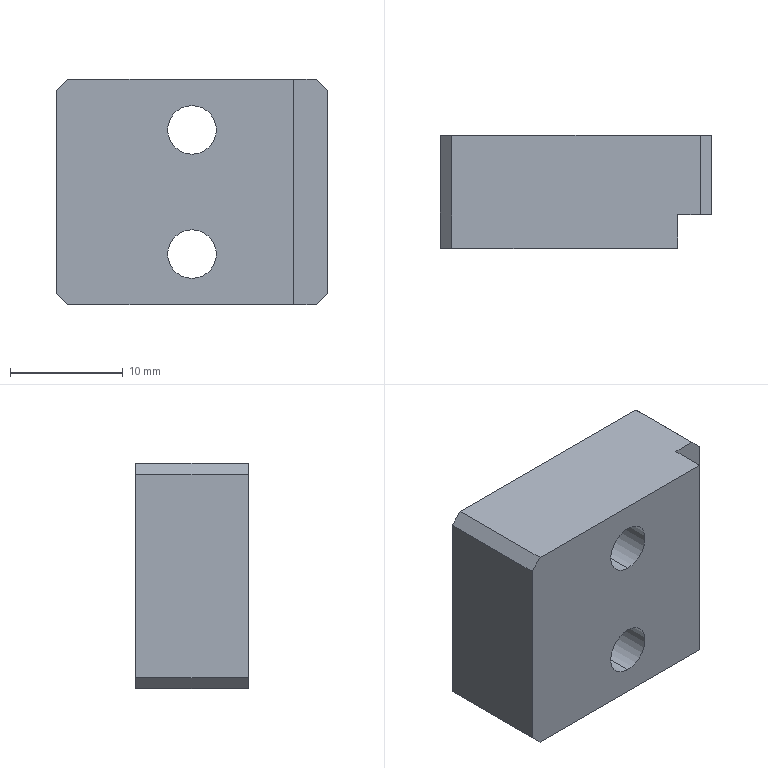Part | STEP file | PN_0059 | 1 solid | 16 faces | box 24 x 10 x 20 mm | volume 4313 mm3 | plane 12 | cylinder 4 | commonest cylinder face diameters 4.3 x4
STEP:
#1=CARTESIAN_POINT('',(0.,0.,0.));
#2=DIRECTION('',(0.,0.,1.));
#3=DIRECTION('',(1.,0.,0.));
#4=AXIS2_PLACEMENT_3D('',#1,#2,#3);
#5=CARTESIAN_POINT('',(0.,0.,7.65));
#6=VERTEX_POINT('',#5);
#7=CARTESIAN_POINT('',(0.,10.,7.65));
#8=VERTEX_POINT('',#7);
#9=CARTESIAN_POINT('',(0.,-43.,7.65));
#10=DIRECTION('',(0.,1.,0.));
#11=VECTOR('',#10,1.);
#12=LINE('',#9,#11);
#13=CARTESIAN_POINT('',(0.,-43.,5.5));
#14=DIRECTION('',(0.,1.,0.));
#15=DIRECTION('',(0.,0.,1.));
#16=AXIS2_PLACEMENT_3D('',#13,#14,#15);
#17=CYLINDRICAL_SURFACE('',#16,2.15);
#18=CARTESIAN_POINT('',(6.283,0.));
#19=DIRECTION('',(0.,1.));
#20=VECTOR('',#19,1.);
#21=LINE('',#18,#20);
#22=(GEOMETRIC_REPRESENTATION_CONTEXT(2)PARAMETRIC_REPRESENTATION_CONTEXT()REPRESENTATION_CONTEXT('',''));
#23=DEFINITIONAL_REPRESENTATION('',(#21),#22);
#24=PCURVE('',#17,#23);
#25=CARTESIAN_POINT('',(0.,-43.,5.5));
#26=DIRECTION('',(0.,1.,0.));
#27=DIRECTION('',(0.,0.,1.));
#28=AXIS2_PLACEMENT_3D('',#25,#26,#27);
#29=CYLINDRICAL_SURFACE('',#28,2.15);
#30=CARTESIAN_POINT('',(0.,0.));
#31=DIRECTION('',(0.,1.));
#32=VECTOR('',#31,1.);
#33=LINE('',#30,#32);
#34=(GEOMETRIC_REPRESENTATION_CONTEXT(2)PARAMETRIC_REPRESENTATION_CONTEXT()REPRESENTATION_CONTEXT('',''));
#35=DEFINITIONAL_REPRESENTATION('',(#33),#34);
#36=PCURVE('',#29,#35);
#37=SURFACE_CURVE('',#12,(#24,#36),.PCURVE_S1.);
#38=EDGE_CURVE('',#6,#8,#37,.T.);
#39=ORIENTED_EDGE('',*,*,#38,.T.);
#40=CARTESIAN_POINT('',(0.,10.,3.35));
#41=VERTEX_POINT('',#40);
#42=CARTESIAN_POINT('',(0.,10.,5.5));
#43=DIRECTION('',(0.,1.,0.));
#44=DIRECTION('',(0.,0.,1.));
#45=AXIS2_PLACEMENT_3D('',#42,#43,#44);
#46=CIRCLE('',#45,2.15);
#47=CARTESIAN_POINT('',(0.,53.));
#48=DIRECTION('',(1.,0.));
#49=VECTOR('',#48,1.);
#50=LINE('',#47,#49);
#51=(GEOMETRIC_REPRESENTATION_CONTEXT(2)PARAMETRIC_REPRESENTATION_CONTEXT()REPRESENTATION_CONTEXT('',''));
#52=DEFINITIONAL_REPRESENTATION('',(#50),#51);
#53=PCURVE('',#17,#52);
#54=CARTESIAN_POINT('',(0.,10.,0.));
#55=DIRECTION('',(0.,1.,0.));
#56=DIRECTION('',(0.,0.,1.));
#57=AXIS2_PLACEMENT_3D('',#54,#55,#56);
#58=PLANE('',#57);
#59=CARTESIAN_POINT('',(5.5,0.));
#60=DIRECTION('',(1.,0.));
#61=AXIS2_PLACEMENT_2D('',#59,#60);
#62=CIRCLE('',#61,2.15);
#63=(GEOMETRIC_REPRESENTATION_CONTEXT(2)PARAMETRIC_REPRESENTATION_CONTEXT()REPRESENTATION_CONTEXT('',''));
#64=DEFINITIONAL_REPRESENTATION('',(#62),#63);
#65=PCURVE('',#58,#64);
#66=SURFACE_CURVE('',#46,(#53,#65),.PCURVE_S1.);
#67=EDGE_CURVE('',#41,#8,#66,.T.);
#68=ORIENTED_EDGE('',*,*,#67,.F.);
#69=CARTESIAN_POINT('',(0.,0.,3.35));
#70=VERTEX_POINT('',#69);
#71=CARTESIAN_POINT('',(0.,-43.,3.35));
#72=DIRECTION('',(0.,1.,0.));
#73=VECTOR('',#72,1.);
#74=LINE('',#71,#73);
#75=CARTESIAN_POINT('',(3.142,0.));
#76=DIRECTION('',(0.,1.));
#77=VECTOR('',#76,1.);
#78=LINE('',#75,#77);
#79=(GEOMETRIC_REPRESENTATION_CONTEXT(2)PARAMETRIC_REPRESENTATION_CONTEXT()REPRESENTATION_CONTEXT('',''));
#80=DEFINITIONAL_REPRESENTATION('',(#78),#79);
#81=PCURVE('',#17,#80);
#82=CARTESIAN_POINT('',(3.142,0.));
#83=DIRECTION('',(0.,1.));
#84=VECTOR('',#83,1.);
#85=LINE('',#82,#84);
#86=(GEOMETRIC_REPRESENTATION_CONTEXT(2)PARAMETRIC_REPRESENTATION_CONTEXT()REPRESENTATION_CONTEXT('',''));
#87=DEFINITIONAL_REPRESENTATION('',(#85),#86);
#88=PCURVE('',#29,#87);
#89=SURFACE_CURVE('',#74,(#81,#88),.PCURVE_S1.);
#90=EDGE_CURVE('',#70,#41,#89,.T.);
#91=ORIENTED_EDGE('',*,*,#90,.F.);
#92=CARTESIAN_POINT('',(0.,0.,5.5));
#93=DIRECTION('',(0.,1.,0.));
#94=DIRECTION('',(0.,0.,1.));
#95=AXIS2_PLACEMENT_3D('',#92,#93,#94);
#96=CIRCLE('',#95,2.15);
#97=CARTESIAN_POINT('',(0.,43.));
#98=DIRECTION('',(1.,0.));
#99=VECTOR('',#98,1.);
#100=LINE('',#97,#99);
#101=(GEOMETRIC_REPRESENTATION_CONTEXT(2)PARAMETRIC_REPRESENTATION_CONTEXT()REPRESENTATION_CONTEXT('',''));
#102=DEFINITIONAL_REPRESENTATION('',(#100),#101);
#103=PCURVE('',#17,#102);
#104=CARTESIAN_POINT('',(0.,0.,0.));
#105=DIRECTION('',(0.,1.,0.));
#106=DIRECTION('',(0.,0.,1.));
#107=AXIS2_PLACEMENT_3D('',#104,#105,#106);
#108=PLANE('',#107);
#109=CARTESIAN_POINT('',(5.5,0.));
#110=DIRECTION('',(1.,0.));
#111=AXIS2_PLACEMENT_2D('',#109,#110);
#112=CIRCLE('',#111,2.15);
#113=(GEOMETRIC_REPRESENTATION_CONTEXT(2)PARAMETRIC_REPRESENTATION_CONTEXT()REPRESENTATION_CONTEXT('',''));
#114=DEFINITIONAL_REPRESENTATION('',(#112),#113);
#115=PCURVE('',#108,#114);
#116=SURFACE_CURVE('',#96,(#103,#115),.PCURVE_S1.);
#117=EDGE_CURVE('',#70,#6,#116,.T.);
#118=ORIENTED_EDGE('',*,*,#117,.T.);
#119=EDGE_LOOP('',(#39,#68,#91,#118));
#120=FACE_BOUND('',#119,.F.);
#121=ADVANCED_FACE('',(#120),#17,.F.);
#122=CARTESIAN_POINT('',(0.,0.,-3.35));
#123=VERTEX_POINT('',#122);
#124=CARTESIAN_POINT('',(0.,10.,-3.35));
#125=VERTEX_POINT('',#124);
#126=CARTESIAN_POINT('',(0.,-43.,-3.35));
#127=DIRECTION('',(0.,1.,0.));
#128=VECTOR('',#127,1.);
#129=LINE('',#126,#128);
#130=CARTESIAN_POINT('',(0.,-43.,-5.5));
#131=DIRECTION('',(0.,1.,0.));
#132=DIRECTION('',(0.,0.,1.));
#133=AXIS2_PLACEMENT_3D('',#130,#131,#132);
#134=CYLINDRICAL_SURFACE('',#133,2.15);
#135=CARTESIAN_POINT('',(6.283,0.));
#136=DIRECTION('',(0.,1.));
#137=VECTOR('',#136,1.);
#138=LINE('',#135,#137);
#139=(GEOMETRIC_REPRESENTATION_CONTEXT(2)PARAMETRIC_REPRESENTATION_CONTEXT()REPRESENTATION_CONTEXT('',''));
#140=DEFINITIONAL_REPRESENTATION('',(#138),#139);
#141=PCURVE('',#134,#140);
#142=CARTESIAN_POINT('',(0.,-43.,-5.5));
#143=DIRECTION('',(0.,1.,0.));
#144=DIRECTION('',(0.,0.,1.));
#145=AXIS2_PLACEMENT_3D('',#142,#143,#144);
#146=CYLINDRICAL_SURFACE('',#145,2.15);
#147=CARTESIAN_POINT('',(0.,0.));
#148=DIRECTION('',(0.,1.));
#149=VECTOR('',#148,1.);
#150=LINE('',#147,#149);
#151=(GEOMETRIC_REPRESENTATION_CONTEXT(2)PARAMETRIC_REPRESENTATION_CONTEXT()REPRESENTATION_CONTEXT('',''));
#152=DEFINITIONAL_REPRESENTATION('',(#150),#151);
#153=PCURVE('',#146,#152);
#154=SURFACE_CURVE('',#129,(#141,#153),.PCURVE_S1.);
#155=EDGE_CURVE('',#123,#125,#154,.T.);
#156=ORIENTED_EDGE('',*,*,#155,.T.);
#157=CARTESIAN_POINT('',(0.,10.,-7.65));
#158=VERTEX_POINT('',#157);
#159=CARTESIAN_POINT('',(0.,10.,-5.5));
#160=DIRECTION('',(0.,1.,0.));
#161=DIRECTION('',(0.,0.,1.));
#162=AXIS2_PLACEMENT_3D('',#159,#160,#161);
#163=CIRCLE('',#162,2.15);
#164=CARTESIAN_POINT('',(0.,53.));
#165=DIRECTION('',(1.,0.));
#166=VECTOR('',#165,1.);
#167=LINE('',#164,#166);
#168=(GEOMETRIC_REPRESENTATION_CONTEXT(2)PARAMETRIC_REPRESENTATION_CONTEXT()REPRESENTATION_CONTEXT('',''));
#169=DEFINITIONAL_REPRESENTATION('',(#167),#168);
#170=PCURVE('',#134,#169);
#171=CARTESIAN_POINT('',(-5.5,0.));
#172=DIRECTION('',(1.,0.));
#173=AXIS2_PLACEMENT_2D('',#171,#172);
#174=CIRCLE('',#173,2.15);
#175=(GEOMETRIC_REPRESENTATION_CONTEXT(2)PARAMETRIC_REPRESENTATION_CONTEXT()REPRESENTATION_CONTEXT('',''));
#176=DEFINITIONAL_REPRESENTATION('',(#174),#175);
#177=PCURVE('',#58,#176);
#178=SURFACE_CURVE('',#163,(#170,#177),.PCURVE_S1.);
#179=EDGE_CURVE('',#158,#125,#178,.T.);
#180=ORIENTED_EDGE('',*,*,#179,.F.);
#181=CARTESIAN_POINT('',(0.,0.,-7.65));
#182=VERTEX_POINT('',#181);
#183=CARTESIAN_POINT('',(0.,-43.,-7.65));
#184=DIRECTION('',(0.,1.,0.));
#185=VECTOR('',#184,1.);
#186=LINE('',#183,#185);
#187=CARTESIAN_POINT('',(3.142,0.));
#188=DIRECTION('',(0.,1.));
#189=VECTOR('',#188,1.);
#190=LINE('',#187,#189);
#191=(GEOMETRIC_REPRESENTATION_CONTEXT(2)PARAMETRIC_REPRESENTATION_CONTEXT()REPRESENTATION_CONTEXT('',''));
#192=DEFINITIONAL_REPRESENTATION('',(#190),#191);
#193=PCURVE('',#134,#192);
#194=CARTESIAN_POINT('',(3.142,0.));
#195=DIRECTION('',(0.,1.));
#196=VECTOR('',#195,1.);
#197=LINE('',#194,#196);
#198=(GEOMETRIC_REPRESENTATION_CONTEXT(2)PARAMETRIC_REPRESENTATION_CONTEXT()REPRESENTATION_CONTEXT('',''));
#199=DEFINITIONAL_REPRESENTATION('',(#197),#198);
#200=PCURVE('',#146,#199);
#201=SURFACE_CURVE('',#186,(#193,#200),.PCURVE_S1.);
#202=EDGE_CURVE('',#182,#158,#201,.T.);
#203=ORIENTED_EDGE('',*,*,#202,.F.);
#204=CARTESIAN_POINT('',(0.,0.,-5.5));
#205=DIRECTION('',(0.,1.,0.));
#206=DIRECTION('',(0.,0.,1.));
#207=AXIS2_PLACEMENT_3D('',#204,#205,#206);
#208=CIRCLE('',#207,2.15);
#209=CARTESIAN_POINT('',(0.,43.));
#210=DIRECTION('',(1.,0.));
#211=VECTOR('',#210,1.);
#212=LINE('',#209,#211);
#213=(GEOMETRIC_REPRESENTATION_CONTEXT(2)PARAMETRIC_REPRESENTATION_CONTEXT()REPRESENTATION_CONTEXT('',''));
#214=DEFINITIONAL_REPRESENTATION('',(#212),#213);
#215=PCURVE('',#134,#214);
#216=CARTESIAN_POINT('',(-5.5,0.));
#217=DIRECTION('',(1.,0.));
#218=AXIS2_PLACEMENT_2D('',#216,#217);
#219=CIRCLE('',#218,2.15);
#220=(GEOMETRIC_REPRESENTATION_CONTEXT(2)PARAMETRIC_REPRESENTATION_CONTEXT()REPRESENTATION_CONTEXT('',''));
#221=DEFINITIONAL_REPRESENTATION('',(#219),#220);
#222=PCURVE('',#108,#221);
#223=SURFACE_CURVE('',#208,(#215,#222),.PCURVE_S1.);
#224=EDGE_CURVE('',#182,#123,#223,.T.);
#225=ORIENTED_EDGE('',*,*,#224,.T.);
#226=EDGE_LOOP('',(#156,#180,#203,#225));
#227=FACE_BOUND('',#226,.F.);
#228=ADVANCED_FACE('',(#227),#134,.F.);
#229=CARTESIAN_POINT('',(12.,3.,-9.));
#230=VERTEX_POINT('',#229);
#231=CARTESIAN_POINT('',(12.,3.,9.));
#232=VERTEX_POINT('',#231);
#233=CARTESIAN_POINT('',(12.,3.,-29.));
#234=DIRECTION('',(0.,0.,1.));
#235=VECTOR('',#234,1.);
#236=LINE('',#233,#235);
#237=CARTESIAN_POINT('',(12.,10.,-10.));
#238=DIRECTION('',(-1.,0.,0.));
#239=DIRECTION('',(0.,0.,1.));
#240=AXIS2_PLACEMENT_3D('',#237,#238,#239);
#241=PLANE('',#240);
#242=CARTESIAN_POINT('',(-19.,-7.));
#243=DIRECTION('',(1.,0.));
#244=VECTOR('',#243,1.);
#245=LINE('',#242,#244);
#246=(GEOMETRIC_REPRESENTATION_CONTEXT(2)PARAMETRIC_REPRESENTATION_CONTEXT()REPRESENTATION_CONTEXT('',''));
#247=DEFINITIONAL_REPRESENTATION('',(#245),#246);
#248=PCURVE('',#241,#247);
#249=CARTESIAN_POINT('',(12.,3.,-29.));
#250=DIRECTION('',(0.,1.,0.));
#251=DIRECTION('',(-1.,0.,0.));
#252=AXIS2_PLACEMENT_3D('',#249,#250,#251);
#253=PLANE('',#252);
#254=CARTESIAN_POINT('',(0.,0.));
#255=DIRECTION('',(0.,1.));
#256=VECTOR('',#255,1.);
#257=LINE('',#254,#256);
#258=(GEOMETRIC_REPRESENTATION_CONTEXT(2)PARAMETRIC_REPRESENTATION_CONTEXT()REPRESENTATION_CONTEXT('',''));
#259=DEFINITIONAL_REPRESENTATION('',(#257),#258);
#260=PCURVE('',#253,#259);
#261=SURFACE_CURVE('',#236,(#248,#260),.PCURVE_S1.);
#262=EDGE_CURVE('',#230,#232,#261,.T.);
#263=ORIENTED_EDGE('',*,*,#262,.F.);
#264=CARTESIAN_POINT('',(12.,10.,-9.));
#265=VERTEX_POINT('',#264);
#266=CARTESIAN_POINT('',(12.,10.,-9.));
#267=DIRECTION('',(0.,1.,0.));
#268=VECTOR('',#267,1.);
#269=LINE('',#266,#268);
#270=CARTESIAN_POINT('',(1.,0.));
#271=DIRECTION('',(0.,1.));
#272=VECTOR('',#271,1.);
#273=LINE('',#270,#272);
#274=(GEOMETRIC_REPRESENTATION_CONTEXT(2)PARAMETRIC_REPRESENTATION_CONTEXT()REPRESENTATION_CONTEXT('',''));
#275=DEFINITIONAL_REPRESENTATION('',(#273),#274);
#276=PCURVE('',#241,#275);
#277=CARTESIAN_POINT('',(11.,10.,-10.));
#278=DIRECTION('',(-0.7071,0.,0.7071));
#279=DIRECTION('',(0.,-1.,0.));
#280=AXIS2_PLACEMENT_3D('',#277,#278,#279);
#281=PLANE('',#280);
#282=CARTESIAN_POINT('',(0.,1.414));
#283=DIRECTION('',(-1.,0.));
#284=VECTOR('',#283,1.);
#285=LINE('',#282,#284);
#286=(GEOMETRIC_REPRESENTATION_CONTEXT(2)PARAMETRIC_REPRESENTATION_CONTEXT()REPRESENTATION_CONTEXT('',''));
#287=DEFINITIONAL_REPRESENTATION('',(#285),#286);
#288=PCURVE('',#281,#287);
#289=SURFACE_CURVE('',#269,(#276,#288),.PCURVE_S1.);
#290=EDGE_CURVE('',#230,#265,#289,.T.);
#291=ORIENTED_EDGE('',*,*,#290,.T.);
#292=CARTESIAN_POINT('',(12.,10.,9.));
#293=VERTEX_POINT('',#292);
#294=CARTESIAN_POINT('',(12.,10.,-10.));
#295=DIRECTION('',(0.,0.,-1.));
#296=VECTOR('',#295,1.);
#297=LINE('',#294,#296);
#298=CARTESIAN_POINT('',(0.,0.));
#299=DIRECTION('',(-1.,0.));
#300=VECTOR('',#299,1.);
#301=LINE('',#298,#300);
#302=(GEOMETRIC_REPRESENTATION_CONTEXT(2)PARAMETRIC_REPRESENTATION_CONTEXT()REPRESENTATION_CONTEXT('',''));
#303=DEFINITIONAL_REPRESENTATION('',(#301),#302);
#304=PCURVE('',#241,#303);
#305=CARTESIAN_POINT('',(-10.,12.));
#306=DIRECTION('',(-1.,0.));
#307=VECTOR('',#306,1.);
#308=LINE('',#305,#307);
#309=(GEOMETRIC_REPRESENTATION_CONTEXT(2)PARAMETRIC_REPRESENTATION_CONTEXT()REPRESENTATION_CONTEXT('',''));
#310=DEFINITIONAL_REPRESENTATION('',(#308),#309);
#311=PCURVE('',#58,#310);
#312=SURFACE_CURVE('',#297,(#304,#311),.PCURVE_S1.);
#313=EDGE_CURVE('',#293,#265,#312,.T.);
#314=ORIENTED_EDGE('',*,*,#313,.F.);
#315=CARTESIAN_POINT('',(12.,10.,9.));
#316=DIRECTION('',(0.,-1.,0.));
#317=VECTOR('',#316,1.);
#318=LINE('',#315,#317);
#319=CARTESIAN_POINT('',(19.,0.));
#320=DIRECTION('',(0.,-1.));
#321=VECTOR('',#320,1.);
#322=LINE('',#319,#321);
#323=(GEOMETRIC_REPRESENTATION_CONTEXT(2)PARAMETRIC_REPRESENTATION_CONTEXT()REPRESENTATION_CONTEXT('',''));
#324=DEFINITIONAL_REPRESENTATION('',(#322),#323);
#325=PCURVE('',#241,#324);
#326=CARTESIAN_POINT('',(12.,10.,9.));
#327=DIRECTION('',(-0.7071,0.,-0.7071));
#328=DIRECTION('',(0.,-1.,0.));
#329=AXIS2_PLACEMENT_3D('',#326,#327,#328);
#330=PLANE('',#329);
#331=CARTESIAN_POINT('',(0.,0.));
#332=DIRECTION('',(1.,0.));
#333=VECTOR('',#332,1.);
#334=LINE('',#331,#333);
#335=(GEOMETRIC_REPRESENTATION_CONTEXT(2)PARAMETRIC_REPRESENTATION_CONTEXT()REPRESENTATION_CONTEXT('',''));
#336=DEFINITIONAL_REPRESENTATION('',(#334),#335);
#337=PCURVE('',#330,#336);
#338=SURFACE_CURVE('',#318,(#325,#337),.PCURVE_S1.);
#339=EDGE_CURVE('',#293,#232,#338,.T.);
#340=ORIENTED_EDGE('',*,*,#339,.T.);
#341=EDGE_LOOP('',(#263,#291,#314,#340));
#342=FACE_BOUND('',#341,.T.);
#343=ADVANCED_FACE('',(#342),#241,.F.);
#344=CARTESIAN_POINT('',(9.,0.,-10.));
#345=VERTEX_POINT('',#344);
#346=CARTESIAN_POINT('',(-11.,0.,-10.));
#347=VERTEX_POINT('',#346);
#348=CARTESIAN_POINT('',(-12.,0.,-10.));
#349=DIRECTION('',(-1.,0.,0.));
#350=VECTOR('',#349,1.);
#351=LINE('',#348,#350);
#352=CARTESIAN_POINT('',(-12.,10.,-10.));
#353=DIRECTION('',(0.,0.,1.));
#354=DIRECTION('',(1.,0.,0.));
#355=AXIS2_PLACEMENT_3D('',#352,#353,#354);
#356=PLANE('',#355);
#357=CARTESIAN_POINT('',(0.,-10.));
#358=DIRECTION('',(-1.,0.));
#359=VECTOR('',#358,1.);
#360=LINE('',#357,#359);
#361=(GEOMETRIC_REPRESENTATION_CONTEXT(2)PARAMETRIC_REPRESENTATION_CONTEXT()REPRESENTATION_CONTEXT('',''));
#362=DEFINITIONAL_REPRESENTATION('',(#360),#361);
#363=PCURVE('',#356,#362);
#364=CARTESIAN_POINT('',(-10.,-12.));
#365=DIRECTION('',(0.,-1.));
#366=VECTOR('',#365,1.);
#367=LINE('',#364,#366);
#368=(GEOMETRIC_REPRESENTATION_CONTEXT(2)PARAMETRIC_REPRESENTATION_CONTEXT()REPRESENTATION_CONTEXT('',''));
#369=DEFINITIONAL_REPRESENTATION('',(#367),#368);
#370=PCURVE('',#108,#369);
#371=SURFACE_CURVE('',#351,(#363,#370),.PCURVE_S1.);
#372=EDGE_CURVE('',#345,#347,#371,.T.);
#373=ORIENTED_EDGE('',*,*,#372,.T.);
#374=CARTESIAN_POINT('',(-11.,10.,-10.));
#375=VERTEX_POINT('',#374);
#376=CARTESIAN_POINT('',(-11.,10.,-10.));
#377=DIRECTION('',(0.,1.,0.));
#378=VECTOR('',#377,1.);
#379=LINE('',#376,#378);
#380=CARTESIAN_POINT('',(1.,0.));
#381=DIRECTION('',(0.,1.));
#382=VECTOR('',#381,1.);
#383=LINE('',#380,#382);
#384=(GEOMETRIC_REPRESENTATION_CONTEXT(2)PARAMETRIC_REPRESENTATION_CONTEXT()REPRESENTATION_CONTEXT('',''));
#385=DEFINITIONAL_REPRESENTATION('',(#383),#384);
#386=PCURVE('',#356,#385);
#387=CARTESIAN_POINT('',(-12.,10.,-9.));
#388=DIRECTION('',(0.7071,0.,0.7071));
#389=DIRECTION('',(0.,-1.,0.));
#390=AXIS2_PLACEMENT_3D('',#387,#388,#389);
#391=PLANE('',#390);
#392=CARTESIAN_POINT('',(0.,1.414));
#393=DIRECTION('',(-1.,0.));
#394=VECTOR('',#393,1.);
#395=LINE('',#392,#394);
#396=(GEOMETRIC_REPRESENTATION_CONTEXT(2)PARAMETRIC_REPRESENTATION_CONTEXT()REPRESENTATION_CONTEXT('',''));
#397=DEFINITIONAL_REPRESENTATION('',(#395),#396);
#398=PCURVE('',#391,#397);
#399=SURFACE_CURVE('',#379,(#386,#398),.PCURVE_S1.);
#400=EDGE_CURVE('',#347,#375,#399,.T.);
#401=ORIENTED_EDGE('',*,*,#400,.T.);
#402=CARTESIAN_POINT('',(11.,10.,-10.));
#403=VERTEX_POINT('',#402);
#404=CARTESIAN_POINT('',(-12.,10.,-10.));
#405=DIRECTION('',(-1.,0.,0.));
#406=VECTOR('',#405,1.);
#407=LINE('',#404,#406);
#408=CARTESIAN_POINT('',(0.,0.));
#409=DIRECTION('',(-1.,0.));
#410=VECTOR('',#409,1.);
#411=LINE('',#408,#410);
#412=(GEOMETRIC_REPRESENTATION_CONTEXT(2)PARAMETRIC_REPRESENTATION_CONTEXT()REPRESENTATION_CONTEXT('',''));
#413=DEFINITIONAL_REPRESENTATION('',(#411),#412);
#414=PCURVE('',#356,#413);
#415=CARTESIAN_POINT('',(-10.,-12.));
#416=DIRECTION('',(0.,-1.));
#417=VECTOR('',#416,1.);
#418=LINE('',#415,#417);
#419=(GEOMETRIC_REPRESENTATION_CONTEXT(2)PARAMETRIC_REPRESENTATION_CONTEXT()REPRESENTATION_CONTEXT('',''));
#420=DEFINITIONAL_REPRESENTATION('',(#418),#419);
#421=PCURVE('',#58,#420);
#422=SURFACE_CURVE('',#407,(#414,#421),.PCURVE_S1.);
#423=EDGE_CURVE('',#403,#375,#422,.T.);
#424=ORIENTED_EDGE('',*,*,#423,.F.);
#425=CARTESIAN_POINT('',(11.,3.,-10.));
#426=VERTEX_POINT('',#425);
#427=CARTESIAN_POINT('',(11.,10.,-10.));
#428=DIRECTION('',(0.,-1.,0.));
#429=VECTOR('',#428,1.);
#430=LINE('',#427,#429);
#431=CARTESIAN_POINT('',(23.,0.));
#432=DIRECTION('',(0.,-1.));
#433=VECTOR('',#432,1.);
#434=LINE('',#431,#433);
#435=(GEOMETRIC_REPRESENTATION_CONTEXT(2)PARAMETRIC_REPRESENTATION_CONTEXT()REPRESENTATION_CONTEXT('',''));
#436=DEFINITIONAL_REPRESENTATION('',(#434),#435);
#437=PCURVE('',#356,#436);
#438=CARTESIAN_POINT('',(0.,0.));
#439=DIRECTION('',(1.,0.));
#440=VECTOR('',#439,1.);
#441=LINE('',#438,#440);
#442=(GEOMETRIC_REPRESENTATION_CONTEXT(2)PARAMETRIC_REPRESENTATION_CONTEXT()REPRESENTATION_CONTEXT('',''));
#443=DEFINITIONAL_REPRESENTATION('',(#441),#442);
#444=PCURVE('',#281,#443);
#445=SURFACE_CURVE('',#430,(#437,#444),.PCURVE_S1.);
#446=EDGE_CURVE('',#403,#426,#445,.T.);
#447=ORIENTED_EDGE('',*,*,#446,.T.);
#448=CARTESIAN_POINT('',(9.,3.,-10.));
#449=VERTEX_POINT('',#448);
#450=CARTESIAN_POINT('',(-12.,3.,-10.));
#451=DIRECTION('',(-1.,0.,0.));
#452=VECTOR('',#451,1.);
#453=LINE('',#450,#452);
#454=CARTESIAN_POINT('',(0.,-7.));
#455=DIRECTION('',(-1.,0.));
#456=VECTOR('',#455,1.);
#457=LINE('',#454,#456);
#458=(GEOMETRIC_REPRESENTATION_CONTEXT(2)PARAMETRIC_REPRESENTATION_CONTEXT()REPRESENTATION_CONTEXT('',''));
#459=DEFINITIONAL_REPRESENTATION('',(#457),#458);
#460=PCURVE('',#356,#459);
#461=CARTESIAN_POINT('',(24.,19.));
#462=DIRECTION('',(1.,0.));
#463=VECTOR('',#462,1.);
#464=LINE('',#461,#463);
#465=(GEOMETRIC_REPRESENTATION_CONTEXT(2)PARAMETRIC_REPRESENTATION_CONTEXT()REPRESENTATION_CONTEXT('',''));
#466=DEFINITIONAL_REPRESENTATION('',(#464),#465);
#467=PCURVE('',#253,#466);
#468=SURFACE_CURVE('',#453,(#460,#467),.PCURVE_S1.);
#469=EDGE_CURVE('',#426,#449,#468,.T.);
#470=ORIENTED_EDGE('',*,*,#469,.T.);
#471=CARTESIAN_POINT('',(9.,10.,-10.));
#472=DIRECTION('',(0.,-1.,0.));
#473=VECTOR('',#472,1.);
#474=LINE('',#471,#473);
#475=CARTESIAN_POINT('',(21.,0.));
#476=DIRECTION('',(0.,-1.));
#477=VECTOR('',#476,1.);
#478=LINE('',#475,#477);
#479=(GEOMETRIC_REPRESENTATION_CONTEXT(2)PARAMETRIC_REPRESENTATION_CONTEXT()REPRESENTATION_CONTEXT('',''));
#480=DEFINITIONAL_REPRESENTATION('',(#478),#479);
#481=PCURVE('',#356,#480);
#482=CARTESIAN_POINT('',(9.,0.,-29.));
#483=DIRECTION('',(-1.,0.,0.));
#484=DIRECTION('',(0.,0.,1.));
#485=AXIS2_PLACEMENT_3D('',#482,#483,#484);
#486=PLANE('',#485);
#487=CARTESIAN_POINT('',(19.,10.));
#488=DIRECTION('',(0.,-1.));
#489=VECTOR('',#488,1.);
#490=LINE('',#487,#489);
#491=(GEOMETRIC_REPRESENTATION_CONTEXT(2)PARAMETRIC_REPRESENTATION_CONTEXT()REPRESENTATION_CONTEXT('',''));
#492=DEFINITIONAL_REPRESENTATION('',(#490),#491);
#493=PCURVE('',#486,#492);
#494=SURFACE_CURVE('',#474,(#481,#493),.PCURVE_S1.);
#495=EDGE_CURVE('',#449,#345,#494,.T.);
#496=ORIENTED_EDGE('',*,*,#495,.T.);
#497=EDGE_LOOP('',(#373,#401,#424,#447,#470,#496));
#498=FACE_BOUND('',#497,.T.);
#499=ADVANCED_FACE('',(#498),#356,.F.);
#500=CARTESIAN_POINT('',(-12.,10.,-9.));
#501=VERTEX_POINT('',#500);
#502=CARTESIAN_POINT('',(-12.,10.,9.));
#503=VERTEX_POINT('',#502);
#504=CARTESIAN_POINT('',(-12.,10.,-10.));
#505=DIRECTION('',(0.,0.,1.));
#506=VECTOR('',#505,1.);
#507=LINE('',#504,#506);
#508=CARTESIAN_POINT('',(-12.,10.,-10.));
#509=DIRECTION('',(1.,0.,0.));
#510=DIRECTION('',(0.,0.,-1.));
#511=AXIS2_PLACEMENT_3D('',#508,#509,#510);
#512=PLANE('',#511);
#513=CARTESIAN_POINT('',(0.,0.));
#514=DIRECTION('',(-1.,0.));
#515=VECTOR('',#514,1.);
#516=LINE('',#513,#515);
#517=(GEOMETRIC_REPRESENTATION_CONTEXT(2)PARAMETRIC_REPRESENTATION_CONTEXT()REPRESENTATION_CONTEXT('',''));
#518=DEFINITIONAL_REPRESENTATION('',(#516),#517);
#519=PCURVE('',#512,#518);
#520=CARTESIAN_POINT('',(-10.,-12.));
#521=DIRECTION('',(1.,0.));
#522=VECTOR('',#521,1.);
#523=LINE('',#520,#522);
#524=(GEOMETRIC_REPRESENTATION_CONTEXT(2)PARAMETRIC_REPRESENTATION_CONTEXT()REPRESENTATION_CONTEXT('',''));
#525=DEFINITIONAL_REPRESENTATION('',(#523),#524);
#526=PCURVE('',#58,#525);
#527=SURFACE_CURVE('',#507,(#519,#526),.PCURVE_S1.);
#528=EDGE_CURVE('',#501,#503,#527,.T.);
#529=ORIENTED_EDGE('',*,*,#528,.F.);
#530=CARTESIAN_POINT('',(-12.,0.,-9.));
#531=VERTEX_POINT('',#530);
#532=CARTESIAN_POINT('',(-12.,10.,-9.));
#533=DIRECTION('',(0.,-1.,0.));
#534=VECTOR('',#533,1.);
#535=LINE('',#532,#534);
#536=CARTESIAN_POINT('',(-1.,0.));
#537=DIRECTION('',(0.,-1.));
#538=VECTOR('',#537,1.);
#539=LINE('',#536,#538);
#540=(GEOMETRIC_REPRESENTATION_CONTEXT(2)PARAMETRIC_REPRESENTATION_CONTEXT()REPRESENTATION_CONTEXT('',''));
#541=DEFINITIONAL_REPRESENTATION('',(#539),#540);
#542=PCURVE('',#512,#541);
#543=CARTESIAN_POINT('',(0.,0.));
#544=DIRECTION('',(1.,0.));
#545=VECTOR('',#544,1.);
#546=LINE('',#543,#545);
#547=(GEOMETRIC_REPRESENTATION_CONTEXT(2)PARAMETRIC_REPRESENTATION_CONTEXT()REPRESENTATION_CONTEXT('',''));
#548=DEFINITIONAL_REPRESENTATION('',(#546),#547);
#549=PCURVE('',#391,#548);
#550=SURFACE_CURVE('',#535,(#542,#549),.PCURVE_S1.);
#551=EDGE_CURVE('',#501,#531,#550,.T.);
#552=ORIENTED_EDGE('',*,*,#551,.T.);
#553=CARTESIAN_POINT('',(-12.,0.,9.));
#554=VERTEX_POINT('',#553);
#555=CARTESIAN_POINT('',(-12.,0.,-10.));
#556=DIRECTION('',(0.,0.,1.));
#557=VECTOR('',#556,1.);
#558=LINE('',#555,#557);
#559=CARTESIAN_POINT('',(0.,-10.));
#560=DIRECTION('',(-1.,0.));
#561=VECTOR('',#560,1.);
#562=LINE('',#559,#561);
#563=(GEOMETRIC_REPRESENTATION_CONTEXT(2)PARAMETRIC_REPRESENTATION_CONTEXT()REPRESENTATION_CONTEXT('',''));
#564=DEFINITIONAL_REPRESENTATION('',(#562),#563);
#565=PCURVE('',#512,#564);
#566=CARTESIAN_POINT('',(-10.,-12.));
#567=DIRECTION('',(1.,0.));
#568=VECTOR('',#567,1.);
#569=LINE('',#566,#568);
#570=(GEOMETRIC_REPRESENTATION_CONTEXT(2)PARAMETRIC_REPRESENTATION_CONTEXT()REPRESENTATION_CONTEXT('',''));
#571=DEFINITIONAL_REPRESENTATION('',(#569),#570);
#572=PCURVE('',#108,#571);
#573=SURFACE_CURVE('',#558,(#565,#572),.PCURVE_S1.);
#574=EDGE_CURVE('',#531,#554,#573,.T.);
#575=ORIENTED_EDGE('',*,*,#574,.T.);
#576=CARTESIAN_POINT('',(-12.,10.,9.));
#577=DIRECTION('',(0.,1.,0.));
#578=VECTOR('',#577,1.);
#579=LINE('',#576,#578);
#580=CARTESIAN_POINT('',(-19.,0.));
#581=DIRECTION('',(0.,1.));
#582=VECTOR('',#581,1.);
#583=LINE('',#580,#582);
#584=(GEOMETRIC_REPRESENTATION_CONTEXT(2)PARAMETRIC_REPRESENTATION_CONTEXT()REPRESENTATION_CONTEXT('',''));
#585=DEFINITIONAL_REPRESENTATION('',(#583),#584);
#586=PCURVE('',#512,#585);
#587=CARTESIAN_POINT('',(-11.,10.,10.));
#588=DIRECTION('',(0.7071,0.,-0.7071));
#589=DIRECTION('',(0.,-1.,0.));
#590=AXIS2_PLACEMENT_3D('',#587,#588,#589);
#591=PLANE('',#590);
#592=CARTESIAN_POINT('',(0.,1.414));
#593=DIRECTION('',(-1.,0.));
#594=VECTOR('',#593,1.);
#595=LINE('',#592,#594);
#596=(GEOMETRIC_REPRESENTATION_CONTEXT(2)PARAMETRIC_REPRESENTATION_CONTEXT()REPRESENTATION_CONTEXT('',''));
#597=DEFINITIONAL_REPRESENTATION('',(#595),#596);
#598=PCURVE('',#591,#597);
#599=SURFACE_CURVE('',#579,(#586,#598),.PCURVE_S1.);
#600=EDGE_CURVE('',#554,#503,#599,.T.);
#601=ORIENTED_EDGE('',*,*,#600,.T.);
#602=EDGE_LOOP('',(#529,#552,#575,#601));
#603=FACE_BOUND('',#602,.T.);
#604=ADVANCED_FACE('',(#603),#512,.F.);
#605=CARTESIAN_POINT('',(11.,3.,10.));
#606=VERTEX_POINT('',#605);
#607=CARTESIAN_POINT('',(9.,3.,10.));
#608=VERTEX_POINT('',#607);
#609=CARTESIAN_POINT('',(12.,3.,10.));
#610=DIRECTION('',(-1.,0.,0.));
#611=VECTOR('',#610,1.);
#612=LINE('',#609,#611);
#613=CARTESIAN_POINT('',(-12.,10.,10.));
#614=DIRECTION('',(0.,0.,-1.));
#615=DIRECTION('',(-1.,0.,0.));
#616=AXIS2_PLACEMENT_3D('',#613,#614,#615);
#617=PLANE('',#616);
#618=CARTESIAN_POINT('',(-24.,-7.));
#619=DIRECTION('',(1.,0.));
#620=VECTOR('',#619,1.);
#621=LINE('',#618,#620);
#622=(GEOMETRIC_REPRESENTATION_CONTEXT(2)PARAMETRIC_REPRESENTATION_CONTEXT()REPRESENTATION_CONTEXT('',''));
#623=DEFINITIONAL_REPRESENTATION('',(#621),#622);
#624=PCURVE('',#617,#623);
#625=CARTESIAN_POINT('',(0.,39.));
#626=DIRECTION('',(1.,0.));
#627=VECTOR('',#626,1.);
#628=LINE('',#625,#627);
#629=(GEOMETRIC_REPRESENTATION_CONTEXT(2)PARAMETRIC_REPRESENTATION_CONTEXT()REPRESENTATION_CONTEXT('',''));
#630=DEFINITIONAL_REPRESENTATION('',(#628),#629);
#631=PCURVE('',#253,#630);
#632=SURFACE_CURVE('',#612,(#624,#631),.PCURVE_S1.);
#633=EDGE_CURVE('',#606,#608,#632,.T.);
#634=ORIENTED_EDGE('',*,*,#633,.F.);
#635=CARTESIAN_POINT('',(11.,10.,10.));
#636=VERTEX_POINT('',#635);
#637=CARTESIAN_POINT('',(11.,10.,10.));
#638=DIRECTION('',(0.,1.,0.));
#639=VECTOR('',#638,1.);
#640=LINE('',#637,#639);
#641=CARTESIAN_POINT('',(-23.,0.));
#642=DIRECTION('',(0.,1.));
#643=VECTOR('',#642,1.);
#644=LINE('',#641,#643);
#645=(GEOMETRIC_REPRESENTATION_CONTEXT(2)PARAMETRIC_REPRESENTATION_CONTEXT()REPRESENTATION_CONTEXT('',''));
#646=DEFINITIONAL_REPRESENTATION('',(#644),#645);
#647=PCURVE('',#617,#646);
#648=CARTESIAN_POINT('',(0.,1.414));
#649=DIRECTION('',(-1.,0.));
#650=VECTOR('',#649,1.);
#651=LINE('',#648,#650);
#652=(GEOMETRIC_REPRESENTATION_CONTEXT(2)PARAMETRIC_REPRESENTATION_CONTEXT()REPRESENTATION_CONTEXT('',''));
#653=DEFINITIONAL_REPRESENTATION('',(#651),#652);
#654=PCURVE('',#330,#653);
#655=SURFACE_CURVE('',#640,(#647,#654),.PCURVE_S1.);
#656=EDGE_CURVE('',#606,#636,#655,.T.);
#657=ORIENTED_EDGE('',*,*,#656,.T.);
#658=CARTESIAN_POINT('',(-11.,10.,10.));
#659=VERTEX_POINT('',#658);
#660=CARTESIAN_POINT('',(-12.,10.,10.));
#661=DIRECTION('',(1.,0.,0.));
#662=VECTOR('',#661,1.);
#663=LINE('',#660,#662);
#664=CARTESIAN_POINT('',(0.,0.));
#665=DIRECTION('',(-1.,0.));
#666=VECTOR('',#665,1.);
#667=LINE('',#664,#666);
#668=(GEOMETRIC_REPRESENTATION_CONTEXT(2)PARAMETRIC_REPRESENTATION_CONTEXT()REPRESENTATION_CONTEXT('',''));
#669=DEFINITIONAL_REPRESENTATION('',(#667),#668);
#670=PCURVE('',#617,#669);
#671=CARTESIAN_POINT('',(10.,-12.));
#672=DIRECTION('',(0.,1.));
#673=VECTOR('',#672,1.);
#674=LINE('',#671,#673);
#675=(GEOMETRIC_REPRESENTATION_CONTEXT(2)PARAMETRIC_REPRESENTATION_CONTEXT()REPRESENTATION_CONTEXT('',''));
#676=DEFINITIONAL_REPRESENTATION('',(#674),#675);
#677=PCURVE('',#58,#676);
#678=SURFACE_CURVE('',#663,(#670,#677),.PCURVE_S1.);
#679=EDGE_CURVE('',#659,#636,#678,.T.);
#680=ORIENTED_EDGE('',*,*,#679,.F.);
#681=CARTESIAN_POINT('',(-11.,0.,10.));
#682=VERTEX_POINT('',#681);
#683=CARTESIAN_POINT('',(-11.,10.,10.));
#684=DIRECTION('',(0.,-1.,0.));
#685=VECTOR('',#684,1.);
#686=LINE('',#683,#685);
#687=CARTESIAN_POINT('',(-1.,0.));
#688=DIRECTION('',(0.,-1.));
#689=VECTOR('',#688,1.);
#690=LINE('',#687,#689);
#691=(GEOMETRIC_REPRESENTATION_CONTEXT(2)PARAMETRIC_REPRESENTATION_CONTEXT()REPRESENTATION_CONTEXT('',''));
#692=DEFINITIONAL_REPRESENTATION('',(#690),#691);
#693=PCURVE('',#617,#692);
#694=CARTESIAN_POINT('',(0.,0.));
#695=DIRECTION('',(1.,0.));
#696=VECTOR('',#695,1.);
#697=LINE('',#694,#696);
#698=(GEOMETRIC_REPRESENTATION_CONTEXT(2)PARAMETRIC_REPRESENTATION_CONTEXT()REPRESENTATION_CONTEXT('',''));
#699=DEFINITIONAL_REPRESENTATION('',(#697),#698);
#700=PCURVE('',#591,#699);
#701=SURFACE_CURVE('',#686,(#693,#700),.PCURVE_S1.);
#702=EDGE_CURVE('',#659,#682,#701,.T.);
#703=ORIENTED_EDGE('',*,*,#702,.T.);
#704=CARTESIAN_POINT('',(9.,0.,10.));
#705=VERTEX_POINT('',#704);
#706=CARTESIAN_POINT('',(-12.,0.,10.));
#707=DIRECTION('',(1.,0.,0.));
#708=VECTOR('',#707,1.);
#709=LINE('',#706,#708);
#710=CARTESIAN_POINT('',(0.,-10.));
#711=DIRECTION('',(-1.,0.));
#712=VECTOR('',#711,1.);
#713=LINE('',#710,#712);
#714=(GEOMETRIC_REPRESENTATION_CONTEXT(2)PARAMETRIC_REPRESENTATION_CONTEXT()REPRESENTATION_CONTEXT('',''));
#715=DEFINITIONAL_REPRESENTATION('',(#713),#714);
#716=PCURVE('',#617,#715);
#717=CARTESIAN_POINT('',(10.,-12.));
#718=DIRECTION('',(0.,1.));
#719=VECTOR('',#718,1.);
#720=LINE('',#717,#719);
#721=(GEOMETRIC_REPRESENTATION_CONTEXT(2)PARAMETRIC_REPRESENTATION_CONTEXT()REPRESENTATION_CONTEXT('',''));
#722=DEFINITIONAL_REPRESENTATION('',(#720),#721);
#723=PCURVE('',#108,#722);
#724=SURFACE_CURVE('',#709,(#716,#723),.PCURVE_S1.);
#725=EDGE_CURVE('',#682,#705,#724,.T.);
#726=ORIENTED_EDGE('',*,*,#725,.T.);
#727=CARTESIAN_POINT('',(9.,0.,10.));
#728=DIRECTION('',(0.,-1.,0.));
#729=VECTOR('',#728,1.);
#730=LINE('',#727,#729);
#731=CARTESIAN_POINT('',(-21.,-10.));
#732=DIRECTION('',(0.,-1.));
#733=VECTOR('',#732,1.);
#734=LINE('',#731,#733);
#735=(GEOMETRIC_REPRESENTATION_CONTEXT(2)PARAMETRIC_REPRESENTATION_CONTEXT()REPRESENTATION_CONTEXT('',''));
#736=DEFINITIONAL_REPRESENTATION('',(#734),#735);
#737=PCURVE('',#617,#736);
#738=CARTESIAN_POINT('',(39.,0.));
#739=DIRECTION('',(0.,-1.));
#740=VECTOR('',#739,1.);
#741=LINE('',#738,#740);
#742=(GEOMETRIC_REPRESENTATION_CONTEXT(2)PARAMETRIC_REPRESENTATION_CONTEXT()REPRESENTATION_CONTEXT('',''));
#743=DEFINITIONAL_REPRESENTATION('',(#741),#742);
#744=PCURVE('',#486,#743);
#745=SURFACE_CURVE('',#730,(#737,#744),.PCURVE_S1.);
#746=EDGE_CURVE('',#608,#705,#745,.T.);
#747=ORIENTED_EDGE('',*,*,#746,.F.);
#748=EDGE_LOOP('',(#634,#657,#680,#703,#726,#747));
#749=FACE_BOUND('',#748,.T.);
#750=ADVANCED_FACE('',(#749),#617,.F.);
#751=CARTESIAN_POINT('',(0.,10.,5.5));
#752=DIRECTION('',(0.,1.,0.));
#753=DIRECTION('',(0.,0.,1.));
#754=AXIS2_PLACEMENT_3D('',#751,#752,#753);
#755=CIRCLE('',#754,2.15);
#756=CARTESIAN_POINT('',(5.5,0.));
#757=DIRECTION('',(1.,0.));
#758=AXIS2_PLACEMENT_2D('',#756,#757);
#759=CIRCLE('',#758,2.15);
#760=(GEOMETRIC_REPRESENTATION_CONTEXT(2)PARAMETRIC_REPRESENTATION_CONTEXT()REPRESENTATION_CONTEXT('',''));
#761=DEFINITIONAL_REPRESENTATION('',(#759),#760);
#762=PCURVE('',#58,#761);
#763=CARTESIAN_POINT('',(0.,53.));
#764=DIRECTION('',(1.,0.));
#765=VECTOR('',#764,1.);
#766=LINE('',#763,#765);
#767=(GEOMETRIC_REPRESENTATION_CONTEXT(2)PARAMETRIC_REPRESENTATION_CONTEXT()REPRESENTATION_CONTEXT('',''));
#768=DEFINITIONAL_REPRESENTATION('',(#766),#767);
#769=PCURVE('',#29,#768);
#770=SURFACE_CURVE('',#755,(#762,#769),.PCURVE_S1.);
#771=EDGE_CURVE('',#8,#41,#770,.T.);
#772=ORIENTED_EDGE('',*,*,#771,.F.);
#773=ORIENTED_EDGE('',*,*,#67,.F.);
#774=EDGE_LOOP('',(#772,#773));
#775=FACE_BOUND('',#774,.T.);
#776=CARTESIAN_POINT('',(0.,10.,-5.5));
#777=DIRECTION('',(0.,1.,0.));
#778=DIRECTION('',(0.,0.,1.));
#779=AXIS2_PLACEMENT_3D('',#776,#777,#778);
#780=CIRCLE('',#779,2.15);
#781=CARTESIAN_POINT('',(-5.5,0.));
#782=DIRECTION('',(1.,0.));
#783=AXIS2_PLACEMENT_2D('',#781,#782);
#784=CIRCLE('',#783,2.15);
#785=(GEOMETRIC_REPRESENTATION_CONTEXT(2)PARAMETRIC_REPRESENTATION_CONTEXT()REPRESENTATION_CONTEXT('',''));
#786=DEFINITIONAL_REPRESENTATION('',(#784),#785);
#787=PCURVE('',#58,#786);
#788=CARTESIAN_POINT('',(0.,53.));
#789=DIRECTION('',(1.,0.));
#790=VECTOR('',#789,1.);
#791=LINE('',#788,#790);
#792=(GEOMETRIC_REPRESENTATION_CONTEXT(2)PARAMETRIC_REPRESENTATION_CONTEXT()REPRESENTATION_CONTEXT('',''));
#793=DEFINITIONAL_REPRESENTATION('',(#791),#792);
#794=PCURVE('',#146,#793);
#795=SURFACE_CURVE('',#780,(#787,#794),.PCURVE_S1.);
#796=EDGE_CURVE('',#125,#158,#795,.T.);
#797=ORIENTED_EDGE('',*,*,#796,.F.);
#798=ORIENTED_EDGE('',*,*,#179,.F.);
#799=EDGE_LOOP('',(#797,#798));
#800=FACE_BOUND('',#799,.T.);
#801=ORIENTED_EDGE('',*,*,#423,.T.);
#802=CARTESIAN_POINT('',(-10.5,10.,-10.5));
#803=DIRECTION('',(-0.7071,0.,0.7071));
#804=VECTOR('',#803,1.);
#805=LINE('',#802,#804);
#806=CARTESIAN_POINT('',(-10.5,-10.5));
#807=DIRECTION('',(0.7071,-0.7071));
#808=VECTOR('',#807,1.);
#809=LINE('',#806,#808);
#810=(GEOMETRIC_REPRESENTATION_CONTEXT(2)PARAMETRIC_REPRESENTATION_CONTEXT()REPRESENTATION_CONTEXT('',''));
#811=DEFINITIONAL_REPRESENTATION('',(#809),#810);
#812=PCURVE('',#58,#811);
#813=CARTESIAN_POINT('',(0.,2.121));
#814=DIRECTION('',(0.,-1.));
#815=VECTOR('',#814,1.);
#816=LINE('',#813,#815);
#817=(GEOMETRIC_REPRESENTATION_CONTEXT(2)PARAMETRIC_REPRESENTATION_CONTEXT()REPRESENTATION_CONTEXT('',''));
#818=DEFINITIONAL_REPRESENTATION('',(#816),#817);
#819=PCURVE('',#391,#818);
#820=SURFACE_CURVE('',#805,(#812,#819),.PCURVE_S1.);
#821=EDGE_CURVE('',#375,#501,#820,.T.);
#822=ORIENTED_EDGE('',*,*,#821,.T.);
#823=ORIENTED_EDGE('',*,*,#528,.T.);
#824=CARTESIAN_POINT('',(-10.5,10.,10.5));
#825=DIRECTION('',(0.7071,0.,0.7071));
#826=VECTOR('',#825,1.);
#827=LINE('',#824,#826);
#828=CARTESIAN_POINT('',(10.5,-10.5));
#829=DIRECTION('',(0.7071,0.7071));
#830=VECTOR('',#829,1.);
#831=LINE('',#828,#830);
#832=(GEOMETRIC_REPRESENTATION_CONTEXT(2)PARAMETRIC_REPRESENTATION_CONTEXT()REPRESENTATION_CONTEXT('',''));
#833=DEFINITIONAL_REPRESENTATION('',(#831),#832);
#834=PCURVE('',#58,#833);
#835=CARTESIAN_POINT('',(0.,-0.7071));
#836=DIRECTION('',(0.,-1.));
#837=VECTOR('',#836,1.);
#838=LINE('',#835,#837);
#839=(GEOMETRIC_REPRESENTATION_CONTEXT(2)PARAMETRIC_REPRESENTATION_CONTEXT()REPRESENTATION_CONTEXT('',''));
#840=DEFINITIONAL_REPRESENTATION('',(#838),#839);
#841=PCURVE('',#591,#840);
#842=SURFACE_CURVE('',#827,(#834,#841),.PCURVE_S1.);
#843=EDGE_CURVE('',#503,#659,#842,.T.);
#844=ORIENTED_EDGE('',*,*,#843,.T.);
#845=ORIENTED_EDGE('',*,*,#679,.T.);
#846=CARTESIAN_POINT('',(10.5,10.,10.5));
#847=DIRECTION('',(0.7071,0.,-0.7071));
#848=VECTOR('',#847,1.);
#849=LINE('',#846,#848);
#850=CARTESIAN_POINT('',(10.5,10.5));
#851=DIRECTION('',(-0.7071,0.7071));
#852=VECTOR('',#851,1.);
#853=LINE('',#850,#852);
#854=(GEOMETRIC_REPRESENTATION_CONTEXT(2)PARAMETRIC_REPRESENTATION_CONTEXT()REPRESENTATION_CONTEXT('',''));
#855=DEFINITIONAL_REPRESENTATION('',(#853),#854);
#856=PCURVE('',#58,#855);
#857=CARTESIAN_POINT('',(0.,2.121));
#858=DIRECTION('',(0.,-1.));
#859=VECTOR('',#858,1.);
#860=LINE('',#857,#859);
#861=(GEOMETRIC_REPRESENTATION_CONTEXT(2)PARAMETRIC_REPRESENTATION_CONTEXT()REPRESENTATION_CONTEXT('',''));
#862=DEFINITIONAL_REPRESENTATION('',(#860),#861);
#863=PCURVE('',#330,#862);
#864=SURFACE_CURVE('',#849,(#856,#863),.PCURVE_S1.);
#865=EDGE_CURVE('',#636,#293,#864,.T.);
#866=ORIENTED_EDGE('',*,*,#865,.T.);
#867=ORIENTED_EDGE('',*,*,#313,.T.);
#868=CARTESIAN_POINT('',(10.5,10.,-10.5));
#869=DIRECTION('',(-0.7071,0.,-0.7071));
#870=VECTOR('',#869,1.);
#871=LINE('',#868,#870);
#872=CARTESIAN_POINT('',(-10.5,10.5));
#873=DIRECTION('',(-0.7071,-0.7071));
#874=VECTOR('',#873,1.);
#875=LINE('',#872,#874);
#876=(GEOMETRIC_REPRESENTATION_CONTEXT(2)PARAMETRIC_REPRESENTATION_CONTEXT()REPRESENTATION_CONTEXT('',''));
#877=DEFINITIONAL_REPRESENTATION('',(#875),#876);
#878=PCURVE('',#58,#877);
#879=CARTESIAN_POINT('',(0.,-0.7071));
#880=DIRECTION('',(0.,-1.));
#881=VECTOR('',#880,1.);
#882=LINE('',#879,#881);
#883=(GEOMETRIC_REPRESENTATION_CONTEXT(2)PARAMETRIC_REPRESENTATION_CONTEXT()REPRESENTATION_CONTEXT('',''));
#884=DEFINITIONAL_REPRESENTATION('',(#882),#883);
#885=PCURVE('',#281,#884);
#886=SURFACE_CURVE('',#871,(#878,#885),.PCURVE_S1.);
#887=EDGE_CURVE('',#265,#403,#886,.T.);
#888=ORIENTED_EDGE('',*,*,#887,.T.);
#889=EDGE_LOOP('',(#801,#822,#823,#844,#845,#866,#867,#888));
#890=FACE_BOUND('',#889,.T.);
#891=ADVANCED_FACE('',(#775,#800,#890),#58,.T.);
#892=CARTESIAN_POINT('',(0.,0.,5.5));
#893=DIRECTION('',(0.,1.,0.));
#894=DIRECTION('',(0.,0.,1.));
#895=AXIS2_PLACEMENT_3D('',#892,#893,#894);
#896=CIRCLE('',#895,2.15);
#897=CARTESIAN_POINT('',(5.5,0.));
#898=DIRECTION('',(1.,0.));
#899=AXIS2_PLACEMENT_2D('',#897,#898);
#900=CIRCLE('',#899,2.15);
#901=(GEOMETRIC_REPRESENTATION_CONTEXT(2)PARAMETRIC_REPRESENTATION_CONTEXT()REPRESENTATION_CONTEXT('',''));
#902=DEFINITIONAL_REPRESENTATION('',(#900),#901);
#903=PCURVE('',#108,#902);
#904=CARTESIAN_POINT('',(0.,43.));
#905=DIRECTION('',(1.,0.));
#906=VECTOR('',#905,1.);
#907=LINE('',#904,#906);
#908=(GEOMETRIC_REPRESENTATION_CONTEXT(2)PARAMETRIC_REPRESENTATION_CONTEXT()REPRESENTATION_CONTEXT('',''));
#909=DEFINITIONAL_REPRESENTATION('',(#907),#908);
#910=PCURVE('',#29,#909);
#911=SURFACE_CURVE('',#896,(#903,#910),.PCURVE_S1.);
#912=EDGE_CURVE('',#6,#70,#911,.T.);
#913=ORIENTED_EDGE('',*,*,#912,.T.);
#914=ORIENTED_EDGE('',*,*,#117,.T.);
#915=EDGE_LOOP('',(#913,#914));
#916=FACE_BOUND('',#915,.T.);
#917=CARTESIAN_POINT('',(0.,0.,-5.5));
#918=DIRECTION('',(0.,1.,0.));
#919=DIRECTION('',(0.,0.,1.));
#920=AXIS2_PLACEMENT_3D('',#917,#918,#919);
#921=CIRCLE('',#920,2.15);
#922=CARTESIAN_POINT('',(-5.5,0.));
#923=DIRECTION('',(1.,0.));
#924=AXIS2_PLACEMENT_2D('',#922,#923);
#925=CIRCLE('',#924,2.15);
#926=(GEOMETRIC_REPRESENTATION_CONTEXT(2)PARAMETRIC_REPRESENTATION_CONTEXT()REPRESENTATION_CONTEXT('',''));
#927=DEFINITIONAL_REPRESENTATION('',(#925),#926);
#928=PCURVE('',#108,#927);
#929=CARTESIAN_POINT('',(0.,43.));
#930=DIRECTION('',(1.,0.));
#931=VECTOR('',#930,1.);
#932=LINE('',#929,#931);
#933=(GEOMETRIC_REPRESENTATION_CONTEXT(2)PARAMETRIC_REPRESENTATION_CONTEXT()REPRESENTATION_CONTEXT('',''));
#934=DEFINITIONAL_REPRESENTATION('',(#932),#933);
#935=PCURVE('',#146,#934);
#936=SURFACE_CURVE('',#921,(#928,#935),.PCURVE_S1.);
#937=EDGE_CURVE('',#123,#182,#936,.T.);
#938=ORIENTED_EDGE('',*,*,#937,.T.);
#939=ORIENTED_EDGE('',*,*,#224,.T.);
#940=EDGE_LOOP('',(#938,#939));
#941=FACE_BOUND('',#940,.T.);
#942=ORIENTED_EDGE('',*,*,#574,.F.);
#943=CARTESIAN_POINT('',(-12.,0.,-9.));
#944=DIRECTION('',(0.7071,0.,-0.7071));
#945=VECTOR('',#944,1.);
#946=LINE('',#943,#945);
#947=CARTESIAN_POINT('',(-9.,-12.));
#948=DIRECTION('',(-0.7071,0.7071));
#949=VECTOR('',#948,1.);
#950=LINE('',#947,#949);
#951=(GEOMETRIC_REPRESENTATION_CONTEXT(2)PARAMETRIC_REPRESENTATION_CONTEXT()REPRESENTATION_CONTEXT('',''));
#952=DEFINITIONAL_REPRESENTATION('',(#950),#951);
#953=PCURVE('',#108,#952);
#954=CARTESIAN_POINT('',(10.,0.));
#955=DIRECTION('',(0.,1.));
#956=VECTOR('',#955,1.);
#957=LINE('',#954,#956);
#958=(GEOMETRIC_REPRESENTATION_CONTEXT(2)PARAMETRIC_REPRESENTATION_CONTEXT()REPRESENTATION_CONTEXT('',''));
#959=DEFINITIONAL_REPRESENTATION('',(#957),#958);
#960=PCURVE('',#391,#959);
#961=SURFACE_CURVE('',#946,(#953,#960),.PCURVE_S1.);
#962=EDGE_CURVE('',#531,#347,#961,.T.);
#963=ORIENTED_EDGE('',*,*,#962,.T.);
#964=ORIENTED_EDGE('',*,*,#372,.F.);
#965=CARTESIAN_POINT('',(9.,0.,0.));
#966=DIRECTION('',(0.,0.,1.));
#967=VECTOR('',#966,1.);
#968=LINE('',#965,#967);
#969=CARTESIAN_POINT('',(0.,9.));
#970=DIRECTION('',(1.,0.));
#971=VECTOR('',#970,1.);
#972=LINE('',#969,#971);
#973=(GEOMETRIC_REPRESENTATION_CONTEXT(2)PARAMETRIC_REPRESENTATION_CONTEXT()REPRESENTATION_CONTEXT('',''));
#974=DEFINITIONAL_REPRESENTATION('',(#972),#973);
#975=PCURVE('',#108,#974);
#976=CARTESIAN_POINT('',(29.,0.));
#977=DIRECTION('',(1.,0.));
#978=VECTOR('',#977,1.);
#979=LINE('',#976,#978);
#980=(GEOMETRIC_REPRESENTATION_CONTEXT(2)PARAMETRIC_REPRESENTATION_CONTEXT()REPRESENTATION_CONTEXT('',''));
#981=DEFINITIONAL_REPRESENTATION('',(#979),#980);
#982=PCURVE('',#486,#981);
#983=SURFACE_CURVE('',#968,(#975,#982),.PCURVE_S1.);
#984=EDGE_CURVE('',#345,#705,#983,.T.);
#985=ORIENTED_EDGE('',*,*,#984,.T.);
#986=ORIENTED_EDGE('',*,*,#725,.F.);
#987=CARTESIAN_POINT('',(-11.,0.,10.));
#988=DIRECTION('',(-0.7071,0.,-0.7071));
#989=VECTOR('',#988,1.);
#990=LINE('',#987,#989);
#991=CARTESIAN_POINT('',(10.,-11.));
#992=DIRECTION('',(-0.7071,-0.7071));
#993=VECTOR('',#992,1.);
#994=LINE('',#991,#993);
#995=(GEOMETRIC_REPRESENTATION_CONTEXT(2)PARAMETRIC_REPRESENTATION_CONTEXT()REPRESENTATION_CONTEXT('',''));
#996=DEFINITIONAL_REPRESENTATION('',(#994),#995);
#997=PCURVE('',#108,#996);
#998=CARTESIAN_POINT('',(10.,0.));
#999=DIRECTION('',(0.,1.));
#1000=VECTOR('',#999,1.);
#1001=LINE('',#998,#1000);
#1002=(GEOMETRIC_REPRESENTATION_CONTEXT(2)PARAMETRIC_REPRESENTATION_CONTEXT()REPRESENTATION_CONTEXT('',''));
#1003=DEFINITIONAL_REPRESENTATION('',(#1001),#1002);
#1004=PCURVE('',#591,#1003);
#1005=SURFACE_CURVE('',#990,(#997,#1004),.PCURVE_S1.);
#1006=EDGE_CURVE('',#682,#554,#1005,.T.);
#1007=ORIENTED_EDGE('',*,*,#1006,.T.);
#1008=EDGE_LOOP('',(#942,#963,#964,#985,#986,#1007));
#1009=FACE_BOUND('',#1008,.T.);
#1010=ADVANCED_FACE('',(#916,#941,#1009),#108,.F.);
#1011=ORIENTED_EDGE('',*,*,#469,.F.);
#1012=CARTESIAN_POINT('',(11.,3.,-10.));
#1013=DIRECTION('',(0.7071,0.,0.7071));
#1014=VECTOR('',#1013,1.);
#1015=LINE('',#1012,#1014);
#1016=CARTESIAN_POINT('',(1.,19.));
#1017=DIRECTION('',(-0.7071,0.7071));
#1018=VECTOR('',#1017,1.);
#1019=LINE('',#1016,#1018);
#1020=(GEOMETRIC_REPRESENTATION_CONTEXT(2)PARAMETRIC_REPRESENTATION_CONTEXT()REPRESENTATION_CONTEXT('',''));
#1021=DEFINITIONAL_REPRESENTATION('',(#1019),#1020);
#1022=PCURVE('',#253,#1021);
#1023=CARTESIAN_POINT('',(7.,0.));
#1024=DIRECTION('',(0.,1.));
#1025=VECTOR('',#1024,1.);
#1026=LINE('',#1023,#1025);
#1027=(GEOMETRIC_REPRESENTATION_CONTEXT(2)PARAMETRIC_REPRESENTATION_CONTEXT()REPRESENTATION_CONTEXT('',''));
#1028=DEFINITIONAL_REPRESENTATION('',(#1026),#1027);
#1029=PCURVE('',#281,#1028);
#1030=SURFACE_CURVE('',#1015,(#1022,#1029),.PCURVE_S1.);
#1031=EDGE_CURVE('',#426,#230,#1030,.T.);
#1032=ORIENTED_EDGE('',*,*,#1031,.T.);
#1033=ORIENTED_EDGE('',*,*,#262,.T.);
#1034=CARTESIAN_POINT('',(12.,3.,9.));
#1035=DIRECTION('',(-0.7071,0.,0.7071));
#1036=VECTOR('',#1035,1.);
#1037=LINE('',#1034,#1036);
#1038=CARTESIAN_POINT('',(0.,38.));
#1039=DIRECTION('',(0.7071,0.7071));
#1040=VECTOR('',#1039,1.);
#1041=LINE('',#1038,#1040);
#1042=(GEOMETRIC_REPRESENTATION_CONTEXT(2)PARAMETRIC_REPRESENTATION_CONTEXT()REPRESENTATION_CONTEXT('',''));
#1043=DEFINITIONAL_REPRESENTATION('',(#1041),#1042);
#1044=PCURVE('',#253,#1043);
#1045=CARTESIAN_POINT('',(7.,0.));
#1046=DIRECTION('',(0.,1.));
#1047=VECTOR('',#1046,1.);
#1048=LINE('',#1045,#1047);
#1049=(GEOMETRIC_REPRESENTATION_CONTEXT(2)PARAMETRIC_REPRESENTATION_CONTEXT()REPRESENTATION_CONTEXT('',''));
#1050=DEFINITIONAL_REPRESENTATION('',(#1048),#1049);
#1051=PCURVE('',#330,#1050);
#1052=SURFACE_CURVE('',#1037,(#1044,#1051),.PCURVE_S1.);
#1053=EDGE_CURVE('',#232,#606,#1052,.T.);
#1054=ORIENTED_EDGE('',*,*,#1053,.T.);
#1055=ORIENTED_EDGE('',*,*,#633,.T.);
#1056=CARTESIAN_POINT('',(9.,3.,-29.));
#1057=DIRECTION('',(0.,0.,1.));
#1058=VECTOR('',#1057,1.);
#1059=LINE('',#1056,#1058);
#1060=CARTESIAN_POINT('',(3.,0.));
#1061=DIRECTION('',(0.,1.));
#1062=VECTOR('',#1061,1.);
#1063=LINE('',#1060,#1062);
#1064=(GEOMETRIC_REPRESENTATION_CONTEXT(2)PARAMETRIC_REPRESENTATION_CONTEXT()REPRESENTATION_CONTEXT('',''));
#1065=DEFINITIONAL_REPRESENTATION('',(#1063),#1064);
#1066=PCURVE('',#253,#1065);
#1067=CARTESIAN_POINT('',(0.,3.));
#1068=DIRECTION('',(1.,0.));
#1069=VECTOR('',#1068,1.);
#1070=LINE('',#1067,#1069);
#1071=(GEOMETRIC_REPRESENTATION_CONTEXT(2)PARAMETRIC_REPRESENTATION_CONTEXT()REPRESENTATION_CONTEXT('',''));
#1072=DEFINITIONAL_REPRESENTATION('',(#1070),#1071);
#1073=PCURVE('',#486,#1072);
#1074=SURFACE_CURVE('',#1059,(#1066,#1073),.PCURVE_S1.);
#1075=EDGE_CURVE('',#449,#608,#1074,.T.);
#1076=ORIENTED_EDGE('',*,*,#1075,.F.);
#1077=EDGE_LOOP('',(#1011,#1032,#1033,#1054,#1055,#1076));
#1078=FACE_BOUND('',#1077,.T.);
#1079=ADVANCED_FACE('',(#1078),#253,.F.);
#1080=ORIENTED_EDGE('',*,*,#1075,.T.);
#1081=ORIENTED_EDGE('',*,*,#746,.T.);
#1082=ORIENTED_EDGE('',*,*,#984,.F.);
#1083=ORIENTED_EDGE('',*,*,#495,.F.);
#1084=EDGE_LOOP('',(#1080,#1081,#1082,#1083));
#1085=FACE_BOUND('',#1084,.T.);
#1086=ADVANCED_FACE('',(#1085),#486,.F.);
#1087=ORIENTED_EDGE('',*,*,#796,.F.);
#1088=ORIENTED_EDGE('',*,*,#155,.F.);
#1089=ORIENTED_EDGE('',*,*,#937,.T.);
#1090=ORIENTED_EDGE('',*,*,#202,.T.);
#1091=EDGE_LOOP('',(#1087,#1088,#1089,#1090));
#1092=FACE_BOUND('',#1091,.F.);
#1093=ADVANCED_FACE('',(#1092),#146,.F.);
#1094=ORIENTED_EDGE('',*,*,#771,.F.);
#1095=ORIENTED_EDGE('',*,*,#38,.F.);
#1096=ORIENTED_EDGE('',*,*,#912,.T.);
#1097=ORIENTED_EDGE('',*,*,#90,.T.);
#1098=EDGE_LOOP('',(#1094,#1095,#1096,#1097));
#1099=FACE_BOUND('',#1098,.F.);
#1100=ADVANCED_FACE('',(#1099),#29,.F.);
#1101=ORIENTED_EDGE('',*,*,#821,.F.);
#1102=ORIENTED_EDGE('',*,*,#400,.F.);
#1103=ORIENTED_EDGE('',*,*,#962,.F.);
#1104=ORIENTED_EDGE('',*,*,#551,.F.);
#1105=EDGE_LOOP('',(#1101,#1102,#1103,#1104));
#1106=FACE_BOUND('',#1105,.T.);
#1107=ADVANCED_FACE('',(#1106),#391,.F.);
#1108=ORIENTED_EDGE('',*,*,#887,.F.);
#1109=ORIENTED_EDGE('',*,*,#290,.F.);
#1110=ORIENTED_EDGE('',*,*,#1031,.F.);
#1111=ORIENTED_EDGE('',*,*,#446,.F.);
#1112=EDGE_LOOP('',(#1108,#1109,#1110,#1111));
#1113=FACE_BOUND('',#1112,.T.);
#1114=ADVANCED_FACE('',(#1113),#281,.F.);
#1115=ORIENTED_EDGE('',*,*,#865,.F.);
#1116=ORIENTED_EDGE('',*,*,#656,.F.);
#1117=ORIENTED_EDGE('',*,*,#1053,.F.);
#1118=ORIENTED_EDGE('',*,*,#339,.F.);
#1119=EDGE_LOOP('',(#1115,#1116,#1117,#1118));
#1120=FACE_BOUND('',#1119,.T.);
#1121=ADVANCED_FACE('',(#1120),#330,.F.);
#1122=ORIENTED_EDGE('',*,*,#843,.F.);
#1123=ORIENTED_EDGE('',*,*,#600,.F.);
#1124=ORIENTED_EDGE('',*,*,#1006,.F.);
#1125=ORIENTED_EDGE('',*,*,#702,.F.);
#1126=EDGE_LOOP('',(#1122,#1123,#1124,#1125));
#1127=FACE_BOUND('',#1126,.T.);
#1128=ADVANCED_FACE('',(#1127),#591,.F.);
#1129=CLOSED_SHELL('',(#121,#228,#343,#499,#604,#750,#891,#1010,#1079,#1086,#1093,#1100,#1107,#1114,#1121,#1128));
#1130=MANIFOLD_SOLID_BREP('',#1129);
#1131=(LENGTH_UNIT()NAMED_UNIT(*)SI_UNIT(.MILLI.,.METRE.));
#1132=UNCERTAINTY_MEASURE_WITH_UNIT(LENGTH_MEASURE(0.0000001),#1131,'','');
#1133=(NAMED_UNIT(*)PLANE_ANGLE_UNIT()SI_UNIT($,.RADIAN.));
#1134=(NAMED_UNIT(*)SI_UNIT($,.STERADIAN.)SOLID_ANGLE_UNIT());
#1135=(GEOMETRIC_REPRESENTATION_CONTEXT(3)GLOBAL_UNCERTAINTY_ASSIGNED_CONTEXT((#1132))GLOBAL_UNIT_ASSIGNED_CONTEXT((#1131,#1133,#1134))REPRESENTATION_CONTEXT('',''));
#1136=ADVANCED_BREP_SHAPE_REPRESENTATION('',(#4,#1130),#1135);